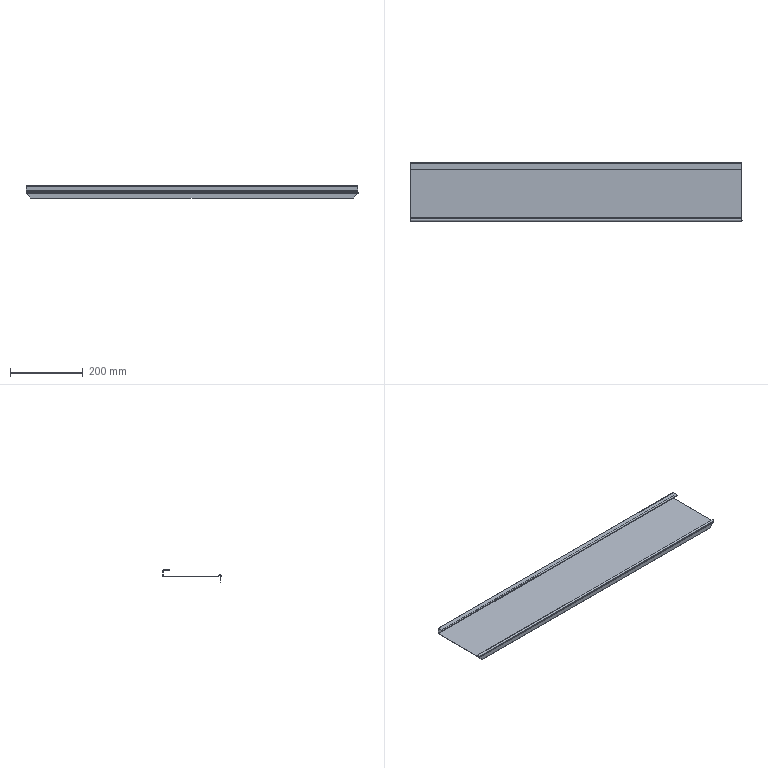Part | SolidWorks | features SM3dBend 4, EdgeFlange 2, FlatPattern 1, Hem 1, SMBaseFlange 1, SheetMetal 1 | 1 solid | 64 faces | box 915 x 160.571 x 33.2 mm | volume 163242 mm3 | plane 48 | cylinder 14 | spline 2 | commonest cylinder face diameters 1 x3 2.6 x3 0.1 x1 1.2 x1 1.7 x1 2.8 x1